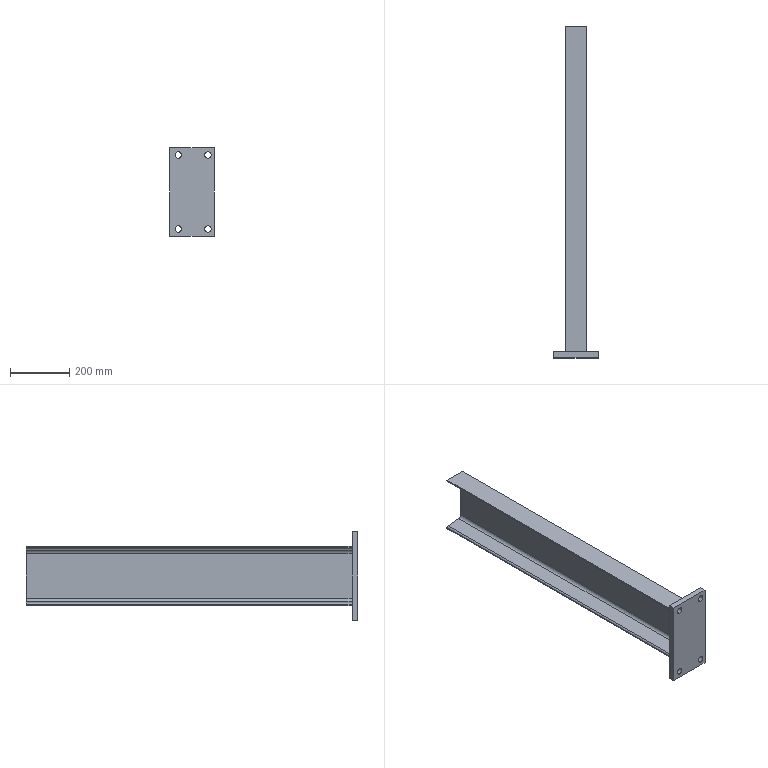Part | SolidWorks | features HoleWzd 1, ICE 1, MirrorPattern 1, WeldMemberFeat 1, WeldmentFeature 1 | 2 solids | 28 faces | box 150 x 1120 x 300 mm | volume 4040615 mm3 | plane 16 | cylinder 12 | commonest cylinder face diameters 22 x10 11 x2
STEP:
#1=CARTESIAN_POINT('',(-73.,588.71,-200.));
#2=VERTEX_POINT('',#1);
#3=CARTESIAN_POINT('',(0.,588.71,-200.));
#4=VERTEX_POINT('',#3);
#5=CARTESIAN_POINT('',(0.,588.71,-200.));
#6=DIRECTION('',(1.,0.,0.));
#7=VECTOR('',#6,1000.);
#8=LINE('',#5,#7);
#9=EDGE_CURVE('',#2,#4,#8,.T.);
#10=ORIENTED_EDGE('',*,*,#9,.T.);
#11=CARTESIAN_POINT('',(0.,-511.29,-200.));
#12=VERTEX_POINT('',#11);
#13=CARTESIAN_POINT('',(0.,-511.29,-200.));
#14=DIRECTION('',(0.,1.,0.));
#15=VECTOR('',#14,1000.);
#16=LINE('',#13,#15);
#17=EDGE_CURVE('',#12,#4,#16,.T.);
#18=ORIENTED_EDGE('',*,*,#17,.F.);
#19=CARTESIAN_POINT('',(-73.,-511.29,-200.));
#20=VERTEX_POINT('',#19);
#21=CARTESIAN_POINT('',(0.,-511.29,-200.));
#22=DIRECTION('',(1.,0.,0.));
#23=VECTOR('',#22,1000.);
#24=LINE('',#21,#23);
#25=EDGE_CURVE('',#20,#12,#24,.T.);
#26=ORIENTED_EDGE('',*,*,#25,.F.);
#27=CARTESIAN_POINT('',(-73.,-511.29,-200.));
#28=DIRECTION('',(0.,1.,0.));
#29=VECTOR('',#28,1000.);
#30=LINE('',#27,#29);
#31=EDGE_CURVE('',#20,#2,#30,.T.);
#32=ORIENTED_EDGE('',*,*,#31,.T.);
#33=EDGE_LOOP('',(#10,#18,#26,#32));
#34=FACE_OUTER_BOUND('',#33,.T.);
#35=CARTESIAN_POINT('',(0.,-511.29,-200.));
#36=DIRECTION('',(0.,0.,1.));
#37=DIRECTION('',(1.,0.,0.));
#38=AXIS2_PLACEMENT_3D('',#35,#36,#37);
#39=PLANE('',#38);
#40=ADVANCED_FACE('',(#34),#39,.F.);
#41=CARTESIAN_POINT('',(0.,588.71,0.));
#42=VERTEX_POINT('',#41);
#43=CARTESIAN_POINT('',(0.,588.71,0.));
#44=DIRECTION('',(0.,0.,1.));
#45=VECTOR('',#44,1000.);
#46=LINE('',#43,#45);
#47=EDGE_CURVE('',#4,#42,#46,.T.);
#48=ORIENTED_EDGE('',*,*,#47,.T.);
#49=CARTESIAN_POINT('',(0.,-511.29,0.));
#50=VERTEX_POINT('',#49);
#51=CARTESIAN_POINT('',(0.,-511.29,0.));
#52=DIRECTION('',(0.,1.,0.));
#53=VECTOR('',#52,1000.);
#54=LINE('',#51,#53);
#55=EDGE_CURVE('',#50,#42,#54,.T.);
#56=ORIENTED_EDGE('',*,*,#55,.F.);
#57=CARTESIAN_POINT('',(0.,-511.29,0.));
#58=DIRECTION('',(0.,0.,1.));
#59=VECTOR('',#58,1000.);
#60=LINE('',#57,#59);
#61=EDGE_CURVE('',#12,#50,#60,.T.);
#62=ORIENTED_EDGE('',*,*,#61,.F.);
#63=ORIENTED_EDGE('',*,*,#17,.T.);
#64=EDGE_LOOP('',(#48,#56,#62,#63));
#65=FACE_OUTER_BOUND('',#64,.T.);
#66=CARTESIAN_POINT('',(0.,-511.29,0.));
#67=DIRECTION('',(-1.,0.,0.));
#68=DIRECTION('',(0.,0.,1.));
#69=AXIS2_PLACEMENT_3D('',#66,#67,#68);
#70=PLANE('',#69);
#71=ADVANCED_FACE('',(#65),#70,.F.);
#72=CARTESIAN_POINT('',(-73.,588.71,0.));
#73=VERTEX_POINT('',#72);
#74=CARTESIAN_POINT('',(0.,588.71,0.));
#75=DIRECTION('',(-1.,0.,0.));
#76=VECTOR('',#75,1000.);
#77=LINE('',#74,#76);
#78=EDGE_CURVE('',#42,#73,#77,.T.);
#79=ORIENTED_EDGE('',*,*,#78,.T.);
#80=CARTESIAN_POINT('',(-73.,-511.29,0.));
#81=VERTEX_POINT('',#80);
#82=CARTESIAN_POINT('',(-73.,-511.29,0.));
#83=DIRECTION('',(0.,1.,0.));
#84=VECTOR('',#83,1000.);
#85=LINE('',#82,#84);
#86=EDGE_CURVE('',#81,#73,#85,.T.);
#87=ORIENTED_EDGE('',*,*,#86,.F.);
#88=CARTESIAN_POINT('',(0.,-511.29,0.));
#89=DIRECTION('',(-1.,0.,0.));
#90=VECTOR('',#89,1000.);
#91=LINE('',#88,#90);
#92=EDGE_CURVE('',#50,#81,#91,.T.);
#93=ORIENTED_EDGE('',*,*,#92,.F.);
#94=ORIENTED_EDGE('',*,*,#55,.T.);
#95=EDGE_LOOP('',(#79,#87,#93,#94));
#96=FACE_OUTER_BOUND('',#95,.T.);
#97=CARTESIAN_POINT('',(0.,-511.29,0.));
#98=DIRECTION('',(0.,0.,-1.));
#99=DIRECTION('',(-1.,0.,0.));
#100=AXIS2_PLACEMENT_3D('',#97,#98,#99);
#101=PLANE('',#100);
#102=ADVANCED_FACE('',(#96),#101,.F.);
#103=CARTESIAN_POINT('',(-73.,588.71,-2.723));
#104=VERTEX_POINT('',#103);
#105=CARTESIAN_POINT('',(-73.,588.71,-2.723));
#106=DIRECTION('',(0.,0.,-1.));
#107=VECTOR('',#106,1000.);
#108=LINE('',#105,#107);
#109=EDGE_CURVE('',#73,#104,#108,.T.);
#110=ORIENTED_EDGE('',*,*,#109,.T.);
#111=CARTESIAN_POINT('',(-73.,-511.29,-2.723));
#112=VERTEX_POINT('',#111);
#113=CARTESIAN_POINT('',(-73.,-511.29,-2.723));
#114=DIRECTION('',(0.,1.,0.));
#115=VECTOR('',#114,1000.);
#116=LINE('',#113,#115);
#117=EDGE_CURVE('',#112,#104,#116,.T.);
#118=ORIENTED_EDGE('',*,*,#117,.F.);
#119=CARTESIAN_POINT('',(-73.,-511.29,-2.723));
#120=DIRECTION('',(0.,0.,-1.));
#121=VECTOR('',#120,1000.);
#122=LINE('',#119,#121);
#123=EDGE_CURVE('',#81,#112,#122,.T.);
#124=ORIENTED_EDGE('',*,*,#123,.F.);
#125=ORIENTED_EDGE('',*,*,#86,.T.);
#126=EDGE_LOOP('',(#110,#118,#124,#125));
#127=FACE_OUTER_BOUND('',#126,.T.);
#128=CARTESIAN_POINT('',(-73.,-511.29,-2.723));
#129=DIRECTION('',(1.,0.,0.));
#130=DIRECTION('',(0.,0.,-1.));
#131=AXIS2_PLACEMENT_3D('',#128,#129,#130);
#132=PLANE('',#131);
#133=ADVANCED_FACE('',(#127),#132,.F.);
#134=CARTESIAN_POINT('',(-68.047,588.71,-8.195));
#135=VERTEX_POINT('',#134);
#136=CARTESIAN_POINT('',(-67.5,588.71,-2.723));
#137=DIRECTION('',(0.,-1.,0.));
#138=DIRECTION('',(1.,0.,0.));
#139=AXIS2_PLACEMENT_3D('',#136,#137,#138);
#140=CIRCLE('',#139,5.5);
#141=EDGE_CURVE('',#104,#135,#140,.T.);
#142=ORIENTED_EDGE('',*,*,#141,.T.);
#143=CARTESIAN_POINT('',(-68.047,-511.29,-8.195));
#144=VERTEX_POINT('',#143);
#145=CARTESIAN_POINT('',(-68.047,-511.29,-8.195));
#146=DIRECTION('',(0.,1.,0.));
#147=VECTOR('',#146,1000.);
#148=LINE('',#145,#147);
#149=EDGE_CURVE('',#144,#135,#148,.T.);
#150=ORIENTED_EDGE('',*,*,#149,.F.);
#151=CARTESIAN_POINT('',(-67.5,-511.29,-2.723));
#152=DIRECTION('',(0.,-1.,0.));
#153=DIRECTION('',(1.,0.,0.));
#154=AXIS2_PLACEMENT_3D('',#151,#152,#153);
#155=CIRCLE('',#154,5.5);
#156=EDGE_CURVE('',#112,#144,#155,.T.);
#157=ORIENTED_EDGE('',*,*,#156,.F.);
#158=ORIENTED_EDGE('',*,*,#117,.T.);
#159=EDGE_LOOP('',(#142,#150,#157,#158));
#160=FACE_OUTER_BOUND('',#159,.T.);
#161=CARTESIAN_POINT('',(-67.5,-511.29,-2.723));
#162=DIRECTION('',(0.,1.,0.));
#163=DIRECTION('',(-1.,0.,0.));
#164=AXIS2_PLACEMENT_3D('',#161,#162,#163);
#165=CYLINDRICAL_SURFACE('',#164,5.5);
#166=ADVANCED_FACE('',(#160),#165,.T.);
#167=CARTESIAN_POINT('',(-16.905,588.71,-13.309));
#168=VERTEX_POINT('',#167);
#169=CARTESIAN_POINT('',(-16.905,588.71,-13.309));
#170=DIRECTION('',(0.995,0.,-0.0995));
#171=VECTOR('',#170,1000.);
#172=LINE('',#169,#171);
#173=EDGE_CURVE('',#135,#168,#172,.T.);
#174=ORIENTED_EDGE('',*,*,#173,.T.);
#175=CARTESIAN_POINT('',(-16.905,-511.29,-13.309));
#176=VERTEX_POINT('',#175);
#177=CARTESIAN_POINT('',(-16.905,-511.29,-13.309));
#178=DIRECTION('',(0.,1.,0.));
#179=VECTOR('',#178,1000.);
#180=LINE('',#177,#179);
#181=EDGE_CURVE('',#176,#168,#180,.T.);
#182=ORIENTED_EDGE('',*,*,#181,.F.);
#183=CARTESIAN_POINT('',(-16.905,-511.29,-13.309));
#184=DIRECTION('',(0.995,0.,-0.0995));
#185=VECTOR('',#184,1000.);
#186=LINE('',#183,#185);
#187=EDGE_CURVE('',#144,#176,#186,.T.);
#188=ORIENTED_EDGE('',*,*,#187,.F.);
#189=ORIENTED_EDGE('',*,*,#149,.T.);
#190=EDGE_LOOP('',(#174,#182,#188,#189));
#191=FACE_OUTER_BOUND('',#190,.T.);
#192=CARTESIAN_POINT('',(-16.905,-511.29,-13.309));
#193=DIRECTION('',(0.0995,0.,0.995));
#194=DIRECTION('',(0.995,0.,-0.0995));
#195=AXIS2_PLACEMENT_3D('',#192,#193,#194);
#196=PLANE('',#195);
#197=ADVANCED_FACE('',(#191),#196,.F.);
#198=CARTESIAN_POINT('',(-7.,588.71,-24.255));
#199=VERTEX_POINT('',#198);
#200=CARTESIAN_POINT('',(-18.,588.71,-24.255));
#201=DIRECTION('',(0.,1.,0.));
#202=DIRECTION('',(-1.,0.,0.));
#203=AXIS2_PLACEMENT_3D('',#200,#201,#202);
#204=CIRCLE('',#203,11.);
#205=EDGE_CURVE('',#168,#199,#204,.T.);
#206=ORIENTED_EDGE('',*,*,#205,.T.);
#207=CARTESIAN_POINT('',(-7.,-511.29,-24.255));
#208=VERTEX_POINT('',#207);
#209=CARTESIAN_POINT('',(-7.,-511.29,-24.255));
#210=DIRECTION('',(0.,1.,0.));
#211=VECTOR('',#210,1000.);
#212=LINE('',#209,#211);
#213=EDGE_CURVE('',#208,#199,#212,.T.);
#214=ORIENTED_EDGE('',*,*,#213,.F.);
#215=CARTESIAN_POINT('',(-18.,-511.29,-24.255));
#216=DIRECTION('',(0.,1.,0.));
#217=DIRECTION('',(-1.,0.,0.));
#218=AXIS2_PLACEMENT_3D('',#215,#216,#217);
#219=CIRCLE('',#218,11.);
#220=EDGE_CURVE('',#176,#208,#219,.T.);
#221=ORIENTED_EDGE('',*,*,#220,.F.);
#222=ORIENTED_EDGE('',*,*,#181,.T.);
#223=EDGE_LOOP('',(#206,#214,#221,#222));
#224=FACE_OUTER_BOUND('',#223,.T.);
#225=CARTESIAN_POINT('',(-18.,-511.29,-24.255));
#226=DIRECTION('',(0.,1.,0.));
#227=DIRECTION('',(-1.,0.,0.));
#228=AXIS2_PLACEMENT_3D('',#225,#226,#227);
#229=CYLINDRICAL_SURFACE('',#228,11.);
#230=ADVANCED_FACE('',(#224),#229,.F.);
#231=CARTESIAN_POINT('',(-7.,588.71,-175.745));
#232=VERTEX_POINT('',#231);
#233=CARTESIAN_POINT('',(-7.,588.71,-175.745));
#234=DIRECTION('',(0.,0.,-1.));
#235=VECTOR('',#234,1000.);
#236=LINE('',#233,#235);
#237=EDGE_CURVE('',#199,#232,#236,.T.);
#238=ORIENTED_EDGE('',*,*,#237,.T.);
#239=CARTESIAN_POINT('',(-7.,-511.29,-175.745));
#240=VERTEX_POINT('',#239);
#241=CARTESIAN_POINT('',(-7.,-511.29,-175.745));
#242=DIRECTION('',(0.,1.,0.));
#243=VECTOR('',#242,1000.);
#244=LINE('',#241,#243);
#245=EDGE_CURVE('',#240,#232,#244,.T.);
#246=ORIENTED_EDGE('',*,*,#245,.F.);
#247=CARTESIAN_POINT('',(-7.,-511.29,-175.745));
#248=DIRECTION('',(0.,0.,-1.));
#249=VECTOR('',#248,1000.);
#250=LINE('',#247,#249);
#251=EDGE_CURVE('',#208,#240,#250,.T.);
#252=ORIENTED_EDGE('',*,*,#251,.F.);
#253=ORIENTED_EDGE('',*,*,#213,.T.);
#254=EDGE_LOOP('',(#238,#246,#252,#253));
#255=FACE_OUTER_BOUND('',#254,.T.);
#256=CARTESIAN_POINT('',(-7.,-511.29,-175.745));
#257=DIRECTION('',(1.,0.,0.));
#258=DIRECTION('',(0.,0.,-1.));
#259=AXIS2_PLACEMENT_3D('',#256,#257,#258);
#260=PLANE('',#259);
#261=ADVANCED_FACE('',(#255),#260,.F.);
#262=CARTESIAN_POINT('',(-16.905,588.71,-186.691));
#263=VERTEX_POINT('',#262);
#264=CARTESIAN_POINT('',(-18.,588.71,-175.745));
#265=DIRECTION('',(0.,1.,0.));
#266=DIRECTION('',(-1.,0.,0.));
#267=AXIS2_PLACEMENT_3D('',#264,#265,#266);
#268=CIRCLE('',#267,11.);
#269=EDGE_CURVE('',#232,#263,#268,.T.);
#270=ORIENTED_EDGE('',*,*,#269,.T.);
#271=CARTESIAN_POINT('',(-16.905,-511.29,-186.691));
#272=VERTEX_POINT('',#271);
#273=CARTESIAN_POINT('',(-16.905,-511.29,-186.691));
#274=DIRECTION('',(0.,1.,0.));
#275=VECTOR('',#274,1000.);
#276=LINE('',#273,#275);
#277=EDGE_CURVE('',#272,#263,#276,.T.);
#278=ORIENTED_EDGE('',*,*,#277,.F.);
#279=CARTESIAN_POINT('',(-18.,-511.29,-175.745));
#280=DIRECTION('',(0.,1.,0.));
#281=DIRECTION('',(-1.,0.,0.));
#282=AXIS2_PLACEMENT_3D('',#279,#280,#281);
#283=CIRCLE('',#282,11.);
#284=EDGE_CURVE('',#240,#272,#283,.T.);
#285=ORIENTED_EDGE('',*,*,#284,.F.);
#286=ORIENTED_EDGE('',*,*,#245,.T.);
#287=EDGE_LOOP('',(#270,#278,#285,#286));
#288=FACE_OUTER_BOUND('',#287,.T.);
#289=CARTESIAN_POINT('',(-18.,-511.29,-175.745));
#290=DIRECTION('',(0.,1.,0.));
#291=DIRECTION('',(-1.,0.,0.));
#292=AXIS2_PLACEMENT_3D('',#289,#290,#291);
#293=CYLINDRICAL_SURFACE('',#292,11.);
#294=ADVANCED_FACE('',(#288),#293,.F.);
#295=CARTESIAN_POINT('',(-68.047,588.71,-191.805));
#296=VERTEX_POINT('',#295);
#297=CARTESIAN_POINT('',(-16.905,588.71,-186.691));
#298=DIRECTION('',(-0.995,0.,-0.0995));
#299=VECTOR('',#298,1000.);
#300=LINE('',#297,#299);
#301=EDGE_CURVE('',#263,#296,#300,.T.);
#302=ORIENTED_EDGE('',*,*,#301,.T.);
#303=CARTESIAN_POINT('',(-68.047,-511.29,-191.805));
#304=VERTEX_POINT('',#303);
#305=CARTESIAN_POINT('',(-68.047,-511.29,-191.805));
#306=DIRECTION('',(0.,1.,0.));
#307=VECTOR('',#306,1000.);
#308=LINE('',#305,#307);
#309=EDGE_CURVE('',#304,#296,#308,.T.);
#310=ORIENTED_EDGE('',*,*,#309,.F.);
#311=CARTESIAN_POINT('',(-16.905,-511.29,-186.691));
#312=DIRECTION('',(-0.995,0.,-0.0995));
#313=VECTOR('',#312,1000.);
#314=LINE('',#311,#313);
#315=EDGE_CURVE('',#272,#304,#314,.T.);
#316=ORIENTED_EDGE('',*,*,#315,.F.);
#317=ORIENTED_EDGE('',*,*,#277,.T.);
#318=EDGE_LOOP('',(#302,#310,#316,#317));
#319=FACE_OUTER_BOUND('',#318,.T.);
#320=CARTESIAN_POINT('',(-16.905,-511.29,-186.691));
#321=DIRECTION('',(0.0995,0.,-0.995));
#322=DIRECTION('',(-0.995,0.,-0.0995));
#323=AXIS2_PLACEMENT_3D('',#320,#321,#322);
#324=PLANE('',#323);
#325=ADVANCED_FACE('',(#319),#324,.F.);
#326=CARTESIAN_POINT('',(-73.,588.71,-197.277));
#327=VERTEX_POINT('',#326);
#328=CARTESIAN_POINT('',(-67.5,588.71,-197.277));
#329=DIRECTION('',(0.,-1.,0.));
#330=DIRECTION('',(1.,0.,0.));
#331=AXIS2_PLACEMENT_3D('',#328,#329,#330);
#332=CIRCLE('',#331,5.5);
#333=EDGE_CURVE('',#296,#327,#332,.T.);
#334=ORIENTED_EDGE('',*,*,#333,.T.);
#335=CARTESIAN_POINT('',(-73.,-511.29,-197.277));
#336=VERTEX_POINT('',#335);
#337=CARTESIAN_POINT('',(-73.,-511.29,-197.277));
#338=DIRECTION('',(0.,1.,0.));
#339=VECTOR('',#338,1000.);
#340=LINE('',#337,#339);
#341=EDGE_CURVE('',#336,#327,#340,.T.);
#342=ORIENTED_EDGE('',*,*,#341,.F.);
#343=CARTESIAN_POINT('',(-67.5,-511.29,-197.277));
#344=DIRECTION('',(0.,-1.,0.));
#345=DIRECTION('',(1.,0.,0.));
#346=AXIS2_PLACEMENT_3D('',#343,#344,#345);
#347=CIRCLE('',#346,5.5);
#348=EDGE_CURVE('',#304,#336,#347,.T.);
#349=ORIENTED_EDGE('',*,*,#348,.F.);
#350=ORIENTED_EDGE('',*,*,#309,.T.);
#351=EDGE_LOOP('',(#334,#342,#349,#350));
#352=FACE_OUTER_BOUND('',#351,.T.);
#353=CARTESIAN_POINT('',(-67.5,-511.29,-197.277));
#354=DIRECTION('',(0.,1.,0.));
#355=DIRECTION('',(-1.,0.,0.));
#356=AXIS2_PLACEMENT_3D('',#353,#354,#355);
#357=CYLINDRICAL_SURFACE('',#356,5.5);
#358=ADVANCED_FACE('',(#352),#357,.T.);
#359=CARTESIAN_POINT('',(-73.,588.71,-197.277));
#360=DIRECTION('',(0.,0.,-1.));
#361=VECTOR('',#360,1000.);
#362=LINE('',#359,#361);
#363=EDGE_CURVE('',#327,#2,#362,.T.);
#364=ORIENTED_EDGE('',*,*,#363,.T.);
#365=ORIENTED_EDGE('',*,*,#31,.F.);
#366=CARTESIAN_POINT('',(-73.,-511.29,-197.277));
#367=DIRECTION('',(0.,0.,-1.));
#368=VECTOR('',#367,1000.);
#369=LINE('',#366,#368);
#370=EDGE_CURVE('',#336,#20,#369,.T.);
#371=ORIENTED_EDGE('',*,*,#370,.F.);
#372=ORIENTED_EDGE('',*,*,#341,.T.);
#373=EDGE_LOOP('',(#364,#365,#371,#372));
#374=FACE_OUTER_BOUND('',#373,.T.);
#375=CARTESIAN_POINT('',(-73.,-511.29,-197.277));
#376=DIRECTION('',(1.,0.,0.));
#377=DIRECTION('',(0.,0.,-1.));
#378=AXIS2_PLACEMENT_3D('',#375,#376,#377);
#379=PLANE('',#378);
#380=ADVANCED_FACE('',(#374),#379,.F.);
#381=ORIENTED_EDGE('',*,*,#25,.T.);
#382=ORIENTED_EDGE('',*,*,#61,.T.);
#383=ORIENTED_EDGE('',*,*,#92,.T.);
#384=ORIENTED_EDGE('',*,*,#123,.T.);
#385=ORIENTED_EDGE('',*,*,#156,.T.);
#386=ORIENTED_EDGE('',*,*,#187,.T.);
#387=ORIENTED_EDGE('',*,*,#220,.T.);
#388=ORIENTED_EDGE('',*,*,#251,.T.);
#389=ORIENTED_EDGE('',*,*,#284,.T.);
#390=ORIENTED_EDGE('',*,*,#315,.T.);
#391=ORIENTED_EDGE('',*,*,#348,.T.);
#392=ORIENTED_EDGE('',*,*,#370,.T.);
#393=EDGE_LOOP('',(#381,#382,#383,#384,#385,#386,#387,#388,#389,#390,#391,#392));
#394=FACE_OUTER_BOUND('',#393,.T.);
#395=CARTESIAN_POINT('',(-67.5,-511.29,-197.277));
#396=DIRECTION('',(0.,-1.,0.));
#397=DIRECTION('',(1.,0.,0.));
#398=AXIS2_PLACEMENT_3D('',#395,#396,#397);
#399=PLANE('',#398);
#400=ADVANCED_FACE('',(#394),#399,.T.);
#401=ORIENTED_EDGE('',*,*,#9,.F.);
#402=ORIENTED_EDGE('',*,*,#363,.F.);
#403=ORIENTED_EDGE('',*,*,#333,.F.);
#404=ORIENTED_EDGE('',*,*,#301,.F.);
#405=ORIENTED_EDGE('',*,*,#269,.F.);
#406=ORIENTED_EDGE('',*,*,#237,.F.);
#407=ORIENTED_EDGE('',*,*,#205,.F.);
#408=ORIENTED_EDGE('',*,*,#173,.F.);
#409=ORIENTED_EDGE('',*,*,#141,.F.);
#410=ORIENTED_EDGE('',*,*,#109,.F.);
#411=ORIENTED_EDGE('',*,*,#78,.F.);
#412=ORIENTED_EDGE('',*,*,#47,.F.);
#413=EDGE_LOOP('',(#401,#402,#403,#404,#405,#406,#407,#408,#409,#410,#411,#412));
#414=FACE_OUTER_BOUND('',#413,.T.);
#415=CARTESIAN_POINT('',(-67.5,588.71,-197.277));
#416=DIRECTION('',(0.,-1.,0.));
#417=DIRECTION('',(1.,0.,0.));
#418=AXIS2_PLACEMENT_3D('',#415,#416,#417);
#419=PLANE('',#418);
#420=ADVANCED_FACE('',(#414),#419,.F.);
#421=CLOSED_SHELL('',(#40,#71,#102,#133,#166,#197,#230,#261,#294,#325,#358,#380,#400,#420));
#422=MANIFOLD_SOLID_BREP('',#421);
#423=CARTESIAN_POINT('',(-82.767,-531.29,36.));
#424=VERTEX_POINT('',#423);
#425=CARTESIAN_POINT('',(-82.767,-531.29,14.));
#426=VERTEX_POINT('',#425);
#427=CARTESIAN_POINT('',(-82.767,-531.29,25.));
#428=DIRECTION('',(0.,-1.,0.));
#429=DIRECTION('',(0.,0.,-1.));
#430=AXIS2_PLACEMENT_3D('',#427,#428,#429);
#431=CIRCLE('',#430,11.);
#432=EDGE_CURVE('',#424,#426,#431,.T.);
#433=ORIENTED_EDGE('',*,*,#432,.T.);
#434=CARTESIAN_POINT('',(-82.767,-511.29,14.));
#435=VERTEX_POINT('',#434);
#436=CARTESIAN_POINT('',(-82.767,-511.29,14.));
#437=DIRECTION('',(0.,1.,0.));
#438=VECTOR('',#437,1000.);
#439=LINE('',#436,#438);
#440=EDGE_CURVE('',#426,#435,#439,.T.);
#441=ORIENTED_EDGE('',*,*,#440,.T.);
#442=CARTESIAN_POINT('',(-82.767,-511.29,36.));
#443=VERTEX_POINT('',#442);
#444=CARTESIAN_POINT('',(-82.767,-511.29,25.));
#445=DIRECTION('',(0.,1.,0.));
#446=DIRECTION('',(0.,0.,1.));
#447=AXIS2_PLACEMENT_3D('',#444,#445,#446);
#448=CIRCLE('',#447,11.);
#449=EDGE_CURVE('',#435,#443,#448,.T.);
#450=ORIENTED_EDGE('',*,*,#449,.T.);
#451=CARTESIAN_POINT('',(-82.767,-511.29,36.));
#452=DIRECTION('',(0.,1.,0.));
#453=VECTOR('',#452,1000.);
#454=LINE('',#451,#453);
#455=EDGE_CURVE('',#424,#443,#454,.T.);
#456=ORIENTED_EDGE('',*,*,#455,.F.);
#457=EDGE_LOOP('',(#433,#441,#450,#456));
#458=FACE_OUTER_BOUND('',#457,.T.);
#459=CARTESIAN_POINT('',(-82.767,-511.29,25.));
#460=DIRECTION('',(0.,1.,0.));
#461=DIRECTION('',(0.,0.,1.));
#462=AXIS2_PLACEMENT_3D('',#459,#460,#461);
#463=CYLINDRICAL_SURFACE('',#462,11.);
#464=ADVANCED_FACE('',(#458),#463,.F.);
#465=CARTESIAN_POINT('',(17.233,-531.29,36.));
#466=VERTEX_POINT('',#465);
#467=CARTESIAN_POINT('',(17.233,-531.29,14.));
#468=VERTEX_POINT('',#467);
#469=CARTESIAN_POINT('',(17.233,-531.29,25.));
#470=DIRECTION('',(0.,-1.,0.));
#471=DIRECTION('',(0.,0.,-1.));
#472=AXIS2_PLACEMENT_3D('',#469,#470,#471);
#473=CIRCLE('',#472,11.);
#474=EDGE_CURVE('',#466,#468,#473,.T.);
#475=ORIENTED_EDGE('',*,*,#474,.T.);
#476=CARTESIAN_POINT('',(17.233,-511.29,14.));
#477=VERTEX_POINT('',#476);
#478=CARTESIAN_POINT('',(17.233,-511.29,14.));
#479=DIRECTION('',(0.,1.,0.));
#480=VECTOR('',#479,1000.);
#481=LINE('',#478,#480);
#482=EDGE_CURVE('',#468,#477,#481,.T.);
#483=ORIENTED_EDGE('',*,*,#482,.T.);
#484=CARTESIAN_POINT('',(17.233,-511.29,36.));
#485=VERTEX_POINT('',#484);
#486=CARTESIAN_POINT('',(17.233,-511.29,25.));
#487=DIRECTION('',(0.,1.,0.));
#488=DIRECTION('',(0.,0.,1.));
#489=AXIS2_PLACEMENT_3D('',#486,#487,#488);
#490=CIRCLE('',#489,11.);
#491=EDGE_CURVE('',#477,#485,#490,.T.);
#492=ORIENTED_EDGE('',*,*,#491,.T.);
#493=CARTESIAN_POINT('',(17.233,-511.29,36.));
#494=DIRECTION('',(0.,1.,0.));
#495=VECTOR('',#494,1000.);
#496=LINE('',#493,#495);
#497=EDGE_CURVE('',#466,#485,#496,.T.);
#498=ORIENTED_EDGE('',*,*,#497,.F.);
#499=EDGE_LOOP('',(#475,#483,#492,#498));
#500=FACE_OUTER_BOUND('',#499,.T.);
#501=CARTESIAN_POINT('',(17.233,-511.29,25.));
#502=DIRECTION('',(0.,1.,0.));
#503=DIRECTION('',(0.,0.,1.));
#504=AXIS2_PLACEMENT_3D('',#501,#502,#503);
#505=CYLINDRICAL_SURFACE('',#504,11.);
#506=ADVANCED_FACE('',(#500),#505,.F.);
#507=CARTESIAN_POINT('',(-82.767,-531.29,-214.));
#508=VERTEX_POINT('',#507);
#509=CARTESIAN_POINT('',(-82.767,-531.29,-236.));
#510=VERTEX_POINT('',#509);
#511=CARTESIAN_POINT('',(-82.767,-531.29,-225.));
#512=DIRECTION('',(0.,-1.,0.));
#513=DIRECTION('',(0.,0.,-1.));
#514=AXIS2_PLACEMENT_3D('',#511,#512,#513);
#515=CIRCLE('',#514,11.);
#516=EDGE_CURVE('',#508,#510,#515,.T.);
#517=ORIENTED_EDGE('',*,*,#516,.T.);
#518=CARTESIAN_POINT('',(-82.767,-511.29,-236.));
#519=VERTEX_POINT('',#518);
#520=CARTESIAN_POINT('',(-82.767,-511.29,-236.));
#521=DIRECTION('',(0.,1.,0.));
#522=VECTOR('',#521,1000.);
#523=LINE('',#520,#522);
#524=EDGE_CURVE('',#510,#519,#523,.T.);
#525=ORIENTED_EDGE('',*,*,#524,.T.);
#526=CARTESIAN_POINT('',(-82.767,-511.29,-214.));
#527=VERTEX_POINT('',#526);
#528=CARTESIAN_POINT('',(-82.767,-511.29,-225.));
#529=DIRECTION('',(0.,1.,0.));
#530=DIRECTION('',(0.,0.,1.));
#531=AXIS2_PLACEMENT_3D('',#528,#529,#530);
#532=CIRCLE('',#531,11.);
#533=EDGE_CURVE('',#519,#527,#532,.T.);
#534=ORIENTED_EDGE('',*,*,#533,.T.);
#535=CARTESIAN_POINT('',(-82.767,-511.29,-214.));
#536=DIRECTION('',(0.,1.,0.));
#537=VECTOR('',#536,1000.);
#538=LINE('',#535,#537);
#539=EDGE_CURVE('',#508,#527,#538,.T.);
#540=ORIENTED_EDGE('',*,*,#539,.F.);
#541=EDGE_LOOP('',(#517,#525,#534,#540));
#542=FACE_OUTER_BOUND('',#541,.T.);
#543=CARTESIAN_POINT('',(-82.767,-511.29,-225.));
#544=DIRECTION('',(0.,1.,0.));
#545=DIRECTION('',(0.,0.,1.));
#546=AXIS2_PLACEMENT_3D('',#543,#544,#545);
#547=CYLINDRICAL_SURFACE('',#546,11.);
#548=ADVANCED_FACE('',(#542),#547,.F.);
#549=CARTESIAN_POINT('',(17.233,-531.29,-214.));
#550=VERTEX_POINT('',#549);
#551=CARTESIAN_POINT('',(17.233,-531.29,-236.));
#552=VERTEX_POINT('',#551);
#553=CARTESIAN_POINT('',(17.233,-531.29,-225.));
#554=DIRECTION('',(0.,-1.,0.));
#555=DIRECTION('',(0.,0.,-1.));
#556=AXIS2_PLACEMENT_3D('',#553,#554,#555);
#557=CIRCLE('',#556,11.);
#558=EDGE_CURVE('',#550,#552,#557,.T.);
#559=ORIENTED_EDGE('',*,*,#558,.T.);
#560=CARTESIAN_POINT('',(17.233,-511.29,-236.));
#561=VERTEX_POINT('',#560);
#562=CARTESIAN_POINT('',(17.233,-511.29,-236.));
#563=DIRECTION('',(0.,1.,0.));
#564=VECTOR('',#563,1000.);
#565=LINE('',#562,#564);
#566=EDGE_CURVE('',#552,#561,#565,.T.);
#567=ORIENTED_EDGE('',*,*,#566,.T.);
#568=CARTESIAN_POINT('',(17.233,-511.29,-214.));
#569=VERTEX_POINT('',#568);
#570=CARTESIAN_POINT('',(17.233,-511.29,-225.));
#571=DIRECTION('',(0.,1.,0.));
#572=DIRECTION('',(0.,0.,1.));
#573=AXIS2_PLACEMENT_3D('',#570,#571,#572);
#574=CIRCLE('',#573,11.);
#575=EDGE_CURVE('',#561,#569,#574,.T.);
#576=ORIENTED_EDGE('',*,*,#575,.T.);
#577=CARTESIAN_POINT('',(17.233,-511.29,-214.));
#578=DIRECTION('',(0.,1.,0.));
#579=VECTOR('',#578,1000.);
#580=LINE('',#577,#579);
#581=EDGE_CURVE('',#550,#569,#580,.T.);
#582=ORIENTED_EDGE('',*,*,#581,.F.);
#583=EDGE_LOOP('',(#559,#567,#576,#582));
#584=FACE_OUTER_BOUND('',#583,.T.);
#585=CARTESIAN_POINT('',(17.233,-511.29,-225.));
#586=DIRECTION('',(0.,1.,0.));
#587=DIRECTION('',(0.,0.,1.));
#588=AXIS2_PLACEMENT_3D('',#585,#586,#587);
#589=CYLINDRICAL_SURFACE('',#588,11.);
#590=ADVANCED_FACE('',(#584),#589,.F.);
#591=CARTESIAN_POINT('',(17.233,-511.29,25.));
#592=DIRECTION('',(0.,1.,0.));
#593=DIRECTION('',(0.,0.,1.));
#594=AXIS2_PLACEMENT_3D('',#591,#592,#593);
#595=CIRCLE('',#594,11.);
#596=EDGE_CURVE('',#485,#477,#595,.T.);
#597=ORIENTED_EDGE('',*,*,#596,.F.);
#598=ORIENTED_EDGE('',*,*,#491,.F.);
#599=EDGE_LOOP('',(#597,#598));
#600=FACE_BOUND('',#599,.T.);
#601=CARTESIAN_POINT('',(-82.767,-511.29,-225.));
#602=DIRECTION('',(0.,1.,0.));
#603=DIRECTION('',(0.,0.,1.));
#604=AXIS2_PLACEMENT_3D('',#601,#602,#603);
#605=CIRCLE('',#604,11.);
#606=EDGE_CURVE('',#527,#519,#605,.T.);
#607=ORIENTED_EDGE('',*,*,#606,.F.);
#608=ORIENTED_EDGE('',*,*,#533,.F.);
#609=EDGE_LOOP('',(#607,#608));
#610=FACE_BOUND('',#609,.T.);
#611=CARTESIAN_POINT('',(17.233,-511.29,-225.));
#612=DIRECTION('',(0.,1.,0.));
#613=DIRECTION('',(0.,0.,1.));
#614=AXIS2_PLACEMENT_3D('',#611,#612,#613);
#615=CIRCLE('',#614,11.);
#616=EDGE_CURVE('',#569,#561,#615,.T.);
#617=ORIENTED_EDGE('',*,*,#616,.F.);
#618=ORIENTED_EDGE('',*,*,#575,.F.);
#619=EDGE_LOOP('',(#617,#618));
#620=FACE_BOUND('',#619,.T.);
#621=CARTESIAN_POINT('',(-111.5,-511.29,50.));
#622=VERTEX_POINT('',#621);
#623=CARTESIAN_POINT('',(-111.5,-511.29,-250.));
#624=VERTEX_POINT('',#623);
#625=CARTESIAN_POINT('',(-111.5,-511.29,-250.));
#626=DIRECTION('',(0.,0.,-1.));
#627=VECTOR('',#626,1000.);
#628=LINE('',#625,#627);
#629=EDGE_CURVE('',#622,#624,#628,.T.);
#630=ORIENTED_EDGE('',*,*,#629,.F.);
#631=CARTESIAN_POINT('',(38.5,-511.29,50.));
#632=VERTEX_POINT('',#631);
#633=CARTESIAN_POINT('',(38.5,-511.29,50.));
#634=DIRECTION('',(-1.,0.,0.));
#635=VECTOR('',#634,1000.);
#636=LINE('',#633,#635);
#637=EDGE_CURVE('',#632,#622,#636,.T.);
#638=ORIENTED_EDGE('',*,*,#637,.F.);
#639=CARTESIAN_POINT('',(38.5,-511.29,-250.));
#640=VERTEX_POINT('',#639);
#641=CARTESIAN_POINT('',(38.5,-511.29,-250.));
#642=DIRECTION('',(0.,0.,1.));
#643=VECTOR('',#642,1000.);
#644=LINE('',#641,#643);
#645=EDGE_CURVE('',#640,#632,#644,.T.);
#646=ORIENTED_EDGE('',*,*,#645,.F.);
#647=CARTESIAN_POINT('',(38.5,-511.29,-250.));
#648=DIRECTION('',(1.,0.,0.));
#649=VECTOR('',#648,1000.);
#650=LINE('',#647,#649);
#651=EDGE_CURVE('',#624,#640,#650,.T.);
#652=ORIENTED_EDGE('',*,*,#651,.F.);
#653=EDGE_LOOP('',(#630,#638,#646,#652));
#654=FACE_OUTER_BOUND('',#653,.T.);
#655=CARTESIAN_POINT('',(-82.767,-511.29,25.));
#656=DIRECTION('',(0.,1.,0.));
#657=DIRECTION('',(0.,0.,1.));
#658=AXIS2_PLACEMENT_3D('',#655,#656,#657);
#659=CIRCLE('',#658,11.);
#660=EDGE_CURVE('',#443,#435,#659,.T.);
#661=ORIENTED_EDGE('',*,*,#660,.F.);
#662=ORIENTED_EDGE('',*,*,#449,.F.);
#663=EDGE_LOOP('',(#661,#662));
#664=FACE_BOUND('',#663,.T.);
#665=CARTESIAN_POINT('',(0.,-511.29,0.));
#666=DIRECTION('',(0.,-1.,0.));
#667=DIRECTION('',(0.,0.,-1.));
#668=AXIS2_PLACEMENT_3D('',#665,#666,#667);
#669=PLANE('',#668);
#670=ADVANCED_FACE('',(#600,#610,#620,#654,#664),#669,.F.);
#671=ORIENTED_EDGE('',*,*,#629,.T.);
#672=CARTESIAN_POINT('',(-111.5,-531.29,-250.));
#673=VERTEX_POINT('',#672);
#674=CARTESIAN_POINT('',(-111.5,-531.29,-250.));
#675=DIRECTION('',(0.,1.,0.));
#676=VECTOR('',#675,1000.);
#677=LINE('',#674,#676);
#678=EDGE_CURVE('',#673,#624,#677,.T.);
#679=ORIENTED_EDGE('',*,*,#678,.F.);
#680=CARTESIAN_POINT('',(-111.5,-531.29,50.));
#681=VERTEX_POINT('',#680);
#682=CARTESIAN_POINT('',(-111.5,-531.29,-250.));
#683=DIRECTION('',(0.,0.,-1.));
#684=VECTOR('',#683,1000.);
#685=LINE('',#682,#684);
#686=EDGE_CURVE('',#681,#673,#685,.T.);
#687=ORIENTED_EDGE('',*,*,#686,.F.);
#688=CARTESIAN_POINT('',(-111.5,-531.29,50.));
#689=DIRECTION('',(0.,1.,0.));
#690=VECTOR('',#689,1000.);
#691=LINE('',#688,#690);
#692=EDGE_CURVE('',#681,#622,#691,.T.);
#693=ORIENTED_EDGE('',*,*,#692,.T.);
#694=EDGE_LOOP('',(#671,#679,#687,#693));
#695=FACE_OUTER_BOUND('',#694,.T.);
#696=CARTESIAN_POINT('',(-111.5,-531.29,-250.));
#697=DIRECTION('',(1.,0.,0.));
#698=DIRECTION('',(0.,0.,-1.));
#699=AXIS2_PLACEMENT_3D('',#696,#697,#698);
#700=PLANE('',#699);
#701=ADVANCED_FACE('',(#695),#700,.F.);
#702=ORIENTED_EDGE('',*,*,#651,.T.);
#703=CARTESIAN_POINT('',(38.5,-531.29,-250.));
#704=VERTEX_POINT('',#703);
#705=CARTESIAN_POINT('',(38.5,-531.29,-250.));
#706=DIRECTION('',(0.,1.,0.));
#707=VECTOR('',#706,1000.);
#708=LINE('',#705,#707);
#709=EDGE_CURVE('',#704,#640,#708,.T.);
#710=ORIENTED_EDGE('',*,*,#709,.F.);
#711=CARTESIAN_POINT('',(38.5,-531.29,-250.));
#712=DIRECTION('',(1.,0.,0.));
#713=VECTOR('',#712,1000.);
#714=LINE('',#711,#713);
#715=EDGE_CURVE('',#673,#704,#714,.T.);
#716=ORIENTED_EDGE('',*,*,#715,.F.);
#717=ORIENTED_EDGE('',*,*,#678,.T.);
#718=EDGE_LOOP('',(#702,#710,#716,#717));
#719=FACE_OUTER_BOUND('',#718,.T.);
#720=CARTESIAN_POINT('',(38.5,-531.29,-250.));
#721=DIRECTION('',(0.,0.,1.));
#722=DIRECTION('',(1.,0.,0.));
#723=AXIS2_PLACEMENT_3D('',#720,#721,#722);
#724=PLANE('',#723);
#725=ADVANCED_FACE('',(#719),#724,.F.);
#726=ORIENTED_EDGE('',*,*,#645,.T.);
#727=CARTESIAN_POINT('',(38.5,-531.29,50.));
#728=VERTEX_POINT('',#727);
#729=CARTESIAN_POINT('',(38.5,-531.29,50.));
#730=DIRECTION('',(0.,1.,0.));
#731=VECTOR('',#730,1000.);
#732=LINE('',#729,#731);
#733=EDGE_CURVE('',#728,#632,#732,.T.);
#734=ORIENTED_EDGE('',*,*,#733,.F.);
#735=CARTESIAN_POINT('',(38.5,-531.29,-250.));
#736=DIRECTION('',(0.,0.,1.));
#737=VECTOR('',#736,1000.);
#738=LINE('',#735,#737);
#739=EDGE_CURVE('',#704,#728,#738,.T.);
#740=ORIENTED_EDGE('',*,*,#739,.F.);
#741=ORIENTED_EDGE('',*,*,#709,.T.);
#742=EDGE_LOOP('',(#726,#734,#740,#741));
#743=FACE_OUTER_BOUND('',#742,.T.);
#744=CARTESIAN_POINT('',(38.5,-531.29,-250.));
#745=DIRECTION('',(-1.,0.,0.));
#746=DIRECTION('',(0.,0.,1.));
#747=AXIS2_PLACEMENT_3D('',#744,#745,#746);
#748=PLANE('',#747);
#749=ADVANCED_FACE('',(#743),#748,.F.);
#750=ORIENTED_EDGE('',*,*,#637,.T.);
#751=ORIENTED_EDGE('',*,*,#692,.F.);
#752=CARTESIAN_POINT('',(38.5,-531.29,50.));
#753=DIRECTION('',(-1.,0.,0.));
#754=VECTOR('',#753,1000.);
#755=LINE('',#752,#754);
#756=EDGE_CURVE('',#728,#681,#755,.T.);
#757=ORIENTED_EDGE('',*,*,#756,.F.);
#758=ORIENTED_EDGE('',*,*,#733,.T.);
#759=EDGE_LOOP('',(#750,#751,#757,#758));
#760=FACE_OUTER_BOUND('',#759,.T.);
#761=CARTESIAN_POINT('',(38.5,-531.29,50.));
#762=DIRECTION('',(0.,0.,-1.));
#763=DIRECTION('',(-1.,0.,0.));
#764=AXIS2_PLACEMENT_3D('',#761,#762,#763);
#765=PLANE('',#764);
#766=ADVANCED_FACE('',(#760),#765,.F.);
#767=ORIENTED_EDGE('',*,*,#432,.F.);
#768=CARTESIAN_POINT('',(-82.767,-531.29,25.));
#769=DIRECTION('',(0.,-1.,0.));
#770=DIRECTION('',(0.,0.,-1.));
#771=AXIS2_PLACEMENT_3D('',#768,#769,#770);
#772=CIRCLE('',#771,11.);
#773=EDGE_CURVE('',#426,#424,#772,.T.);
#774=ORIENTED_EDGE('',*,*,#773,.F.);
#775=EDGE_LOOP('',(#767,#774));
#776=FACE_BOUND('',#775,.T.);
#777=ORIENTED_EDGE('',*,*,#474,.F.);
#778=CARTESIAN_POINT('',(17.233,-531.29,25.));
#779=DIRECTION('',(0.,-1.,0.));
#780=DIRECTION('',(0.,0.,-1.));
#781=AXIS2_PLACEMENT_3D('',#778,#779,#780);
#782=CIRCLE('',#781,11.);
#783=EDGE_CURVE('',#468,#466,#782,.T.);
#784=ORIENTED_EDGE('',*,*,#783,.F.);
#785=EDGE_LOOP('',(#777,#784));
#786=FACE_BOUND('',#785,.T.);
#787=ORIENTED_EDGE('',*,*,#516,.F.);
#788=CARTESIAN_POINT('',(-82.767,-531.29,-225.));
#789=DIRECTION('',(0.,-1.,0.));
#790=DIRECTION('',(0.,0.,-1.));
#791=AXIS2_PLACEMENT_3D('',#788,#789,#790);
#792=CIRCLE('',#791,11.);
#793=EDGE_CURVE('',#510,#508,#792,.T.);
#794=ORIENTED_EDGE('',*,*,#793,.F.);
#795=EDGE_LOOP('',(#787,#794));
#796=FACE_BOUND('',#795,.T.);
#797=ORIENTED_EDGE('',*,*,#558,.F.);
#798=CARTESIAN_POINT('',(17.233,-531.29,-225.));
#799=DIRECTION('',(0.,-1.,0.));
#800=DIRECTION('',(0.,0.,-1.));
#801=AXIS2_PLACEMENT_3D('',#798,#799,#800);
#802=CIRCLE('',#801,11.);
#803=EDGE_CURVE('',#552,#550,#802,.T.);
#804=ORIENTED_EDGE('',*,*,#803,.F.);
#805=EDGE_LOOP('',(#797,#804));
#806=FACE_BOUND('',#805,.T.);
#807=ORIENTED_EDGE('',*,*,#686,.T.);
#808=ORIENTED_EDGE('',*,*,#715,.T.);
#809=ORIENTED_EDGE('',*,*,#739,.T.);
#810=ORIENTED_EDGE('',*,*,#756,.T.);
#811=EDGE_LOOP('',(#807,#808,#809,#810));
#812=FACE_OUTER_BOUND('',#811,.T.);
#813=CARTESIAN_POINT('',(0.,-531.29,0.));
#814=DIRECTION('',(0.,-1.,0.));
#815=DIRECTION('',(0.,0.,-1.));
#816=AXIS2_PLACEMENT_3D('',#813,#814,#815);
#817=PLANE('',#816);
#818=ADVANCED_FACE('',(#776,#786,#796,#806,#812),#817,.T.);
#819=ORIENTED_EDGE('',*,*,#566,.F.);
#820=ORIENTED_EDGE('',*,*,#803,.T.);
#821=ORIENTED_EDGE('',*,*,#581,.T.);
#822=ORIENTED_EDGE('',*,*,#616,.T.);
#823=EDGE_LOOP('',(#819,#820,#821,#822));
#824=FACE_OUTER_BOUND('',#823,.T.);
#825=CARTESIAN_POINT('',(17.233,-511.29,-225.));
#826=DIRECTION('',(0.,1.,0.));
#827=DIRECTION('',(0.,0.,1.));
#828=AXIS2_PLACEMENT_3D('',#825,#826,#827);
#829=CYLINDRICAL_SURFACE('',#828,11.);
#830=ADVANCED_FACE('',(#824),#829,.F.);
#831=ORIENTED_EDGE('',*,*,#524,.F.);
#832=ORIENTED_EDGE('',*,*,#793,.T.);
#833=ORIENTED_EDGE('',*,*,#539,.T.);
#834=ORIENTED_EDGE('',*,*,#606,.T.);
#835=EDGE_LOOP('',(#831,#832,#833,#834));
#836=FACE_OUTER_BOUND('',#835,.T.);
#837=CARTESIAN_POINT('',(-82.767,-511.29,-225.));
#838=DIRECTION('',(0.,1.,0.));
#839=DIRECTION('',(0.,0.,1.));
#840=AXIS2_PLACEMENT_3D('',#837,#838,#839);
#841=CYLINDRICAL_SURFACE('',#840,11.);
#842=ADVANCED_FACE('',(#836),#841,.F.);
#843=ORIENTED_EDGE('',*,*,#482,.F.);
#844=ORIENTED_EDGE('',*,*,#783,.T.);
#845=ORIENTED_EDGE('',*,*,#497,.T.);
#846=ORIENTED_EDGE('',*,*,#596,.T.);
#847=EDGE_LOOP('',(#843,#844,#845,#846));
#848=FACE_OUTER_BOUND('',#847,.T.);
#849=CARTESIAN_POINT('',(17.233,-511.29,25.));
#850=DIRECTION('',(0.,1.,0.));
#851=DIRECTION('',(0.,0.,1.));
#852=AXIS2_PLACEMENT_3D('',#849,#850,#851);
#853=CYLINDRICAL_SURFACE('',#852,11.);
#854=ADVANCED_FACE('',(#848),#853,.F.);
#855=ORIENTED_EDGE('',*,*,#440,.F.);
#856=ORIENTED_EDGE('',*,*,#773,.T.);
#857=ORIENTED_EDGE('',*,*,#455,.T.);
#858=ORIENTED_EDGE('',*,*,#660,.T.);
#859=EDGE_LOOP('',(#855,#856,#857,#858));
#860=FACE_OUTER_BOUND('',#859,.T.);
#861=CARTESIAN_POINT('',(-82.767,-511.29,25.));
#862=DIRECTION('',(0.,1.,0.));
#863=DIRECTION('',(0.,0.,1.));
#864=AXIS2_PLACEMENT_3D('',#861,#862,#863);
#865=CYLINDRICAL_SURFACE('',#864,11.);
#866=ADVANCED_FACE('',(#860),#865,.F.);
#867=CLOSED_SHELL('',(#464,#506,#548,#590,#670,#701,#725,#749,#766,#818,#830,#842,#854,#866));
#868=MANIFOLD_SOLID_BREP('',#867);
#869=CARTESIAN_POINT('',(0.,0.,0.));
#870=DIRECTION('',(0.,0.,1.));
#871=DIRECTION('',(1.,0.,0.));
#872=AXIS2_PLACEMENT_3D('',#869,#870,#871);
#873=(LENGTH_UNIT()NAMED_UNIT(*)SI_UNIT(.MILLI.,.METRE.));
#874=UNCERTAINTY_MEASURE_WITH_UNIT(LENGTH_MEASURE(0.00001),#873,'','');
#875=(NAMED_UNIT(*)PLANE_ANGLE_UNIT()SI_UNIT($,.RADIAN.));
#876=(NAMED_UNIT(*)SI_UNIT($,.STERADIAN.)SOLID_ANGLE_UNIT());
#877=(GEOMETRIC_REPRESENTATION_CONTEXT(3)GLOBAL_UNCERTAINTY_ASSIGNED_CONTEXT((#874))GLOBAL_UNIT_ASSIGNED_CONTEXT((#873,#875,#876))REPRESENTATION_CONTEXT('',''));
#878=ADVANCED_BREP_SHAPE_REPRESENTATION('',(#422,#868,#872),#877);